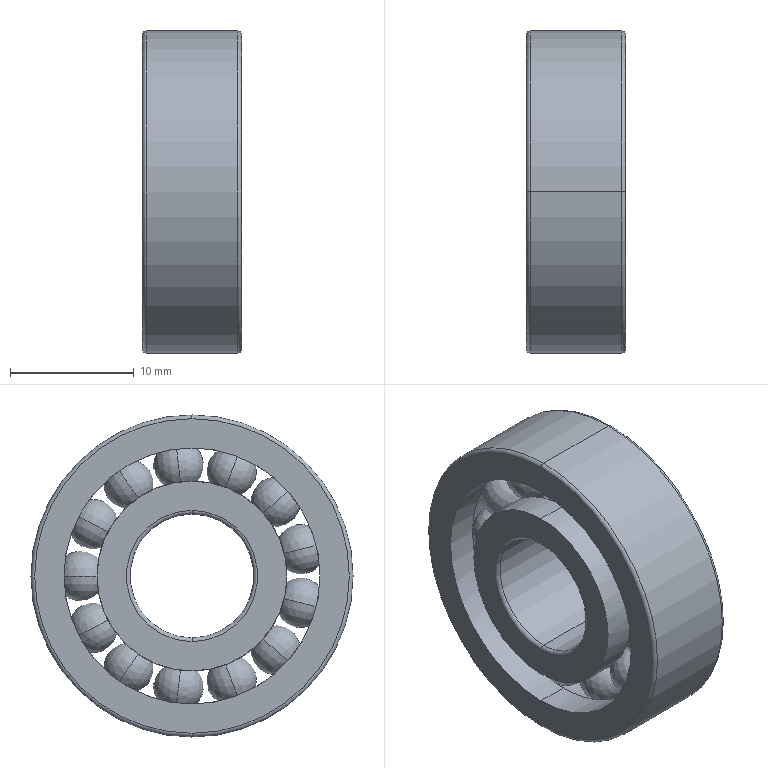Part | NX | 1 solid | 92 faces | box 8 x 26 x 26 mm | volume 2693 mm3 | torus 50 | sphere 26 | cylinder 12 | plane 4 | commonest cylinder face diameters 15.333 x4 20.667 x4 10 x2 26 x2